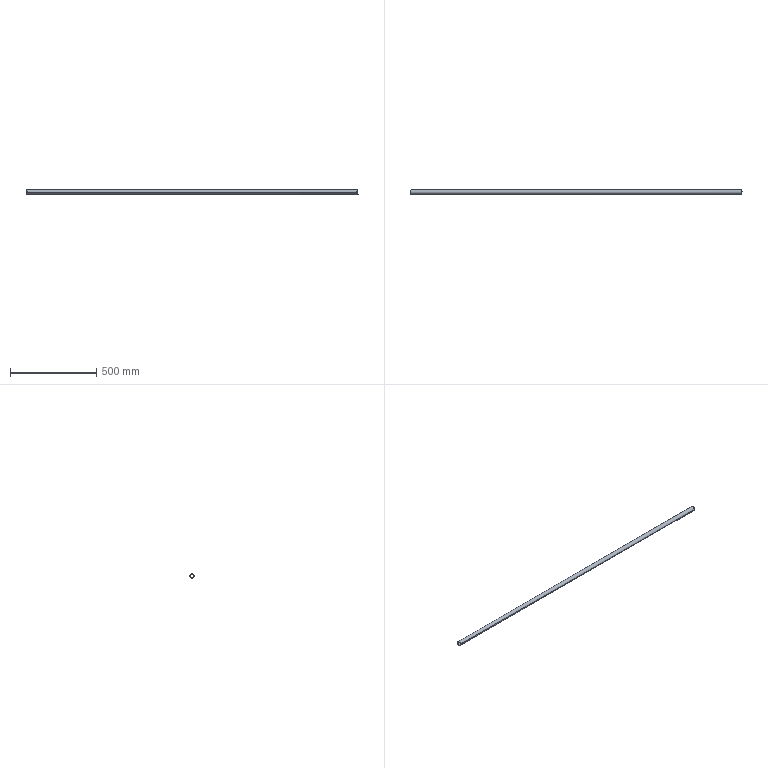Part | NX | features BREP 1 | 1 solid | 7 faces | box 1927 x 25.4 x 25.399 mm | volume 177519 mm3 | cylinder 7 | commonest cylinder face diameters 31.75 x3 22.962 x2 25.4 x2
STEP:
#1=CARTESIAN_POINT('',(956.945,12.7,0.));
#2=VERTEX_POINT('',#1);
#3=CARTESIAN_POINT('',(-956.945,12.7,0.));
#4=VERTEX_POINT('',#3);
#5=CARTESIAN_POINT('',(-956.945,12.7,0.));
#6=DIRECTION('',(1.,0.,0.));
#7=VECTOR('',#6,1000.);
#8=LINE('',#5,#7);
#9=EDGE_CURVE('',#2,#4,#8,.F.);
#10=ORIENTED_EDGE('',*,*,#9,.F.);
#11=CARTESIAN_POINT('',(956.945,-12.7,0.));
#12=VERTEX_POINT('',#11);
#13=CARTESIAN_POINT('',(956.945,12.7,0.));
#14=CARTESIAN_POINT('',(956.945,12.7,-0.8859));
#15=CARTESIAN_POINT('',(957.059,12.563,-2.235));
#16=CARTESIAN_POINT('',(957.402,12.128,-3.814));
#17=CARTESIAN_POINT('',(957.645,11.816,-4.678));
#18=CARTESIAN_POINT('',(957.885,11.505,-5.391));
#19=CARTESIAN_POINT('',(958.046,11.298,-5.808));
#20=CARTESIAN_POINT('',(958.333,10.925,-6.498));
#21=CARTESIAN_POINT('',(958.745,10.381,-7.355));
#22=CARTESIAN_POINT('',(959.259,9.666,-8.259));
#23=CARTESIAN_POINT('',(959.707,9.019,-8.954));
#24=CARTESIAN_POINT('',(960.114,8.412,-9.523));
#25=CARTESIAN_POINT('',(960.378,8.006,-9.864));
#26=CARTESIAN_POINT('',(960.689,7.509,-10.249));
#27=CARTESIAN_POINT('',(960.985,7.02,-10.59));
#28=CARTESIAN_POINT('',(961.44,6.237,-11.079));
#29=CARTESIAN_POINT('',(961.814,5.523,-11.447));
#30=CARTESIAN_POINT('',(962.136,4.844,-11.743));
#31=CARTESIAN_POINT('',(962.319,4.431,-11.906));
#32=CARTESIAN_POINT('',(962.56,3.825,-12.116));
#33=CARTESIAN_POINT('',(962.813,3.091,-12.328));
#34=CARTESIAN_POINT('',(963.166,1.783,-12.612));
#35=CARTESIAN_POINT('',(963.378,0.09483,-12.755));
#36=CARTESIAN_POINT('',(963.175,-1.743,-12.623));
#37=CARTESIAN_POINT('',(962.799,-3.121,-12.324));
#38=CARTESIAN_POINT('',(962.548,-3.837,-12.109));
#39=CARTESIAN_POINT('',(962.397,-4.227,-11.978));
#40=CARTESIAN_POINT('',(962.249,-4.583,-11.845));
#41=CARTESIAN_POINT('',(962.195,-4.704,-11.797));
#42=CARTESIAN_POINT('',(962.075,-4.971,-11.689));
#43=CARTESIAN_POINT('',(961.85,-5.442,-11.482));
#44=CARTESIAN_POINT('',(961.43,-6.257,-11.075));
#45=CARTESIAN_POINT('',(960.884,-7.208,-10.475));
#46=CARTESIAN_POINT('',(960.39,-8.002,-9.875));
#47=CARTESIAN_POINT('',(959.939,-8.674,-9.287));
#48=CARTESIAN_POINT('',(959.623,-9.123,-8.843));
#49=CARTESIAN_POINT('',(959.19,-9.741,-8.171));
#50=CARTESIAN_POINT('',(958.714,-10.403,-7.323));
#51=CARTESIAN_POINT('',(958.211,-11.082,-6.239));
#52=CARTESIAN_POINT('',(957.818,-11.596,-5.231));
#53=CARTESIAN_POINT('',(957.411,-12.117,-3.893));
#54=CARTESIAN_POINT('',(957.057,-12.565,-2.178));
#55=CARTESIAN_POINT('',(956.945,-12.7,-0.8592));
#56=CARTESIAN_POINT('',(956.945,-12.7,0.));
#57=B_SPLINE_CURVE_WITH_KNOTS('',3,(#13,#14,#15,#16,#17,#18,#19,#20,#21,#22,#23,#24,#25,#26,#27,#28,#29,#30,#31,#32,#33,#34,#35,#36,#37,#38,#39,#40,#41,#42,#43,#44,#45,#46,#47,#48,#49,#50,#51,#52,#53,#54,#55,#56),.UNSPECIFIED.,.F.,.F.,(4,1,1,1,1,1,1,1,1,1,1,1,1,1,1,1,1,1,1,1,1,1,1,1,1,1,1,1,1,1,1,1,1,1,1,1,1,1,1,1,1,4),(0.,0.0625,0.09375,0.1094,0.125,0.1406,0.1562,0.1875,0.2188,0.2344,0.25,0.2656,0.2812,0.2969,0.3125,0.3438,0.3594,0.375,0.3906,0.4062,0.4375,0.5,0.5625,0.5938,0.6094,0.6172,0.625,0.6328,0.6406,0.6562,0.6875,0.7188,0.7344,0.75,0.7656,0.7812,0.8125,0.8438,0.875,0.9062,0.9375,1.),.UNSPECIFIED.);
#58=EDGE_CURVE('',#2,#12,#57,.T.);
#59=ORIENTED_EDGE('',*,*,#58,.T.);
#60=CARTESIAN_POINT('',(-956.945,-12.7,0.));
#61=VERTEX_POINT('',#60);
#62=CARTESIAN_POINT('',(-956.945,-12.7,0.));
#63=DIRECTION('',(1.,0.,0.));
#64=VECTOR('',#63,1000.);
#65=LINE('',#62,#64);
#66=EDGE_CURVE('',#12,#61,#65,.F.);
#67=ORIENTED_EDGE('',*,*,#66,.T.);
#68=CARTESIAN_POINT('',(-956.945,-12.7,0.));
#69=CARTESIAN_POINT('',(-956.945,-12.7,-0.876));
#70=CARTESIAN_POINT('',(-957.056,-12.566,-2.209));
#71=CARTESIAN_POINT('',(-957.391,-12.142,-3.77));
#72=CARTESIAN_POINT('',(-957.629,-11.836,-4.625));
#73=CARTESIAN_POINT('',(-957.863,-11.534,-5.328));
#74=CARTESIAN_POINT('',(-958.023,-11.327,-5.75));
#75=CARTESIAN_POINT('',(-958.306,-10.96,-6.438));
#76=CARTESIAN_POINT('',(-958.712,-10.424,-7.292));
#77=CARTESIAN_POINT('',(-959.214,-9.728,-8.186));
#78=CARTESIAN_POINT('',(-959.653,-9.096,-8.874));
#79=CARTESIAN_POINT('',(-960.047,-8.514,-9.432));
#80=CARTESIAN_POINT('',(-960.317,-8.1,-9.787));
#81=CARTESIAN_POINT('',(-960.721,-7.459,-10.293));
#82=CARTESIAN_POINT('',(-961.228,-6.625,-10.856));
#83=CARTESIAN_POINT('',(-961.782,-5.609,-11.412));
#84=CARTESIAN_POINT('',(-962.429,-4.239,-12.016));
#85=CARTESIAN_POINT('',(-963.083,-2.309,-12.552));
#86=CARTESIAN_POINT('',(-963.365,-0.3495,-12.746));
#87=CARTESIAN_POINT('',(-963.225,1.463,-12.659));
#88=CARTESIAN_POINT('',(-962.889,2.82,-12.393));
#89=CARTESIAN_POINT('',(-962.648,3.576,-12.193));
#90=CARTESIAN_POINT('',(-962.397,4.239,-11.976));
#91=CARTESIAN_POINT('',(-962.262,4.554,-11.857));
#92=CARTESIAN_POINT('',(-961.981,5.177,-11.606));
#93=CARTESIAN_POINT('',(-961.559,6.02,-11.206));
#94=CARTESIAN_POINT('',(-961.006,7.006,-10.612));
#95=CARTESIAN_POINT('',(-960.504,7.825,-10.015));
#96=CARTESIAN_POINT('',(-959.916,8.71,-9.271));
#97=CARTESIAN_POINT('',(-959.364,9.497,-8.466));
#98=CARTESIAN_POINT('',(-958.742,10.367,-7.38));
#99=CARTESIAN_POINT('',(-958.222,11.067,-6.267));
#100=CARTESIAN_POINT('',(-957.817,11.596,-5.234));
#101=CARTESIAN_POINT('',(-957.413,12.114,-3.899));
#102=CARTESIAN_POINT('',(-957.057,12.565,-2.18));
#103=CARTESIAN_POINT('',(-956.945,12.7,-0.8602));
#104=CARTESIAN_POINT('',(-956.945,12.7,0.));
#105=B_SPLINE_CURVE_WITH_KNOTS('',3,(#68,#69,#70,#71,#72,#73,#74,#75,#76,#77,#78,#79,#80,#81,#82,#83,#84,#85,#86,#87,#88,#89,#90,#91,#92,#93,#94,#95,#96,#97,#98,#99,#100,#101,#102,#103,#104),.UNSPECIFIED.,.F.,.F.,(4,1,1,1,1,1,1,1,1,1,1,1,1,1,1,1,1,1,1,1,1,1,1,1,1,1,1,1,1,1,1,1,1,1,4),(0.,0.0625,0.09375,0.1094,0.125,0.1406,0.1562,0.1875,0.2188,0.2344,0.25,0.2656,0.2812,0.3125,0.3438,0.375,0.4375,0.5,0.5625,0.5938,0.6094,0.625,0.6406,0.6562,0.6875,0.7188,0.7344,0.75,0.7812,0.8125,0.8438,0.875,0.9062,0.9375,1.),.UNSPECIFIED.);
#106=EDGE_CURVE('',#61,#4,#105,.T.);
#107=ORIENTED_EDGE('',*,*,#106,.T.);
#108=EDGE_LOOP('',(#10,#59,#67,#107));
#109=FACE_BOUND('',#108,.T.);
#110=CARTESIAN_POINT('',(-969.645,0.,0.));
#111=DIRECTION('',(1.,0.,0.));
#112=DIRECTION('',(0.,-1.,0.));
#113=AXIS2_PLACEMENT_3D('',#110,#111,#112);
#114=CYLINDRICAL_SURFACE('',#113,12.7);
#115=ADVANCED_FACE('',(#109),#114,.T.);
#116=CARTESIAN_POINT('',(-956.945,-11.481,0.));
#117=VERTEX_POINT('',#116);
#118=CARTESIAN_POINT('',(-956.945,15.24,0.));
#119=DIRECTION('',(0.,1.,0.));
#120=VECTOR('',#119,1000.);
#121=LINE('',#118,#120);
#122=EDGE_CURVE('',#61,#117,#121,.T.);
#123=ORIENTED_EDGE('',*,*,#122,.F.);
#124=CARTESIAN_POINT('',(-956.945,-12.7,0.));
#125=CARTESIAN_POINT('',(-956.945,-12.7,0.8854));
#126=CARTESIAN_POINT('',(-957.087,-12.525,2.634));
#127=CARTESIAN_POINT('',(-957.769,-11.66,5.253));
#128=CARTESIAN_POINT('',(-958.707,-10.43,7.392));
#129=CARTESIAN_POINT('',(-959.963,-8.668,9.401));
#130=CARTESIAN_POINT('',(-961.232,-6.69,10.895));
#131=CARTESIAN_POINT('',(-962.311,-4.584,11.922));
#132=CARTESIAN_POINT('',(-963.14,-2.186,12.589));
#133=CARTESIAN_POINT('',(-963.377,0.1165,12.759));
#134=CARTESIAN_POINT('',(-963.115,2.222,12.569));
#135=CARTESIAN_POINT('',(-962.125,5.179,11.77));
#136=CARTESIAN_POINT('',(-960.512,7.881,10.216));
#137=CARTESIAN_POINT('',(-958.811,10.298,7.591));
#138=CARTESIAN_POINT('',(-957.826,11.584,5.425));
#139=CARTESIAN_POINT('',(-957.096,12.515,2.72));
#140=CARTESIAN_POINT('',(-956.945,12.7,0.9154));
#141=CARTESIAN_POINT('',(-956.945,12.7,0.));
#142=B_SPLINE_CURVE_WITH_KNOTS('',3,(#124,#125,#126,#127,#128,#129,#130,#131,#132,#133,#134,#135,#136,#137,#138,#139,#140,#141),.UNSPECIFIED.,.F.,.F.,(4,1,1,1,1,1,1,1,1,1,1,1,1,1,1,4),(0.,0.0625,0.125,0.1875,0.25,0.3125,0.375,0.4375,0.5,0.5625,0.625,0.75,0.8125,0.875,0.9375,1.),.UNSPECIFIED.);
#143=EDGE_CURVE('',#4,#61,#142,.F.);
#144=ORIENTED_EDGE('',*,*,#143,.F.);
#145=CARTESIAN_POINT('',(-956.945,11.481,0.));
#146=VERTEX_POINT('',#145);
#147=CARTESIAN_POINT('',(-956.945,15.24,0.));
#148=DIRECTION('',(0.,1.,0.));
#149=VECTOR('',#148,1000.);
#150=LINE('',#147,#149);
#151=EDGE_CURVE('',#146,#4,#150,.T.);
#152=ORIENTED_EDGE('',*,*,#151,.F.);
#153=CARTESIAN_POINT('',(-956.945,11.481,0.));
#154=CARTESIAN_POINT('',(-956.945,11.481,1.594));
#155=CARTESIAN_POINT('',(-957.457,10.786,4.809));
#156=CARTESIAN_POINT('',(-959.008,8.49,7.997));
#157=CARTESIAN_POINT('',(-960.369,5.992,9.887));
#158=CARTESIAN_POINT('',(-961.202,4.,10.834));
#159=CARTESIAN_POINT('',(-961.776,1.843,11.407));
#160=CARTESIAN_POINT('',(-961.915,-0.3564,11.535));
#161=CARTESIAN_POINT('',(-961.674,-2.312,11.31));
#162=CARTESIAN_POINT('',(-960.861,-5.056,10.477));
#163=CARTESIAN_POINT('',(-959.606,-7.456,8.956));
#164=CARTESIAN_POINT('',(-958.332,-9.494,6.599));
#165=CARTESIAN_POINT('',(-957.323,-10.965,3.954));
#166=CARTESIAN_POINT('',(-956.945,-11.481,1.568));
#167=CARTESIAN_POINT('',(-956.945,-11.481,0.));
#168=B_SPLINE_CURVE_WITH_KNOTS('',3,(#153,#154,#155,#156,#157,#158,#159,#160,#161,#162,#163,#164,#165,#166,#167),.UNSPECIFIED.,.F.,.F.,(4,1,1,1,1,1,1,1,1,1,1,1,4),(0.,0.125,0.25,0.3125,0.375,0.4375,0.5,0.5625,0.625,0.75,0.8125,0.875,1.),.UNSPECIFIED.);
#169=EDGE_CURVE('',#117,#146,#168,.F.);
#170=ORIENTED_EDGE('',*,*,#169,.F.);
#171=EDGE_LOOP('',(#123,#144,#152,#170));
#172=FACE_BOUND('',#171,.T.);
#173=CARTESIAN_POINT('',(-972.82,15.24,0.));
#174=DIRECTION('',(0.,1.,0.));
#175=DIRECTION('',(1.,0.,0.));
#176=AXIS2_PLACEMENT_3D('',#173,#174,#175);
#177=CYLINDRICAL_SURFACE('',#176,15.875);
#178=ADVANCED_FACE('',(#172),#177,.F.);
#179=ORIENTED_EDGE('',*,*,#66,.F.);
#180=CARTESIAN_POINT('',(956.945,-12.7,0.));
#181=CARTESIAN_POINT('',(956.945,-12.7,0.8723));
#182=CARTESIAN_POINT('',(957.055,-12.567,2.2));
#183=CARTESIAN_POINT('',(957.387,-12.147,3.754));
#184=CARTESIAN_POINT('',(957.623,-11.844,4.604));
#185=CARTESIAN_POINT('',(957.854,-11.545,5.304));
#186=CARTESIAN_POINT('',(958.014,-11.339,5.726));
#187=CARTESIAN_POINT('',(958.295,-10.975,6.413));
#188=CARTESIAN_POINT('',(958.697,-10.444,7.263));
#189=CARTESIAN_POINT('',(959.194,-9.756,8.152));
#190=CARTESIAN_POINT('',(959.628,-9.132,8.837));
#191=CARTESIAN_POINT('',(960.017,-8.558,9.392));
#192=CARTESIAN_POINT('',(960.286,-8.148,9.746));
#193=CARTESIAN_POINT('',(960.687,-7.515,10.253));
#194=CARTESIAN_POINT('',(961.19,-6.69,10.816));
#195=CARTESIAN_POINT('',(961.743,-5.683,11.375));
#196=CARTESIAN_POINT('',(962.391,-4.33,11.983));
#197=CARTESIAN_POINT('',(963.064,-2.389,12.538));
#198=CARTESIAN_POINT('',(963.362,-0.437,12.744));
#199=CARTESIAN_POINT('',(963.234,1.414,12.666));
#200=CARTESIAN_POINT('',(962.898,2.789,12.4));
#201=CARTESIAN_POINT('',(962.656,3.554,12.199));
#202=CARTESIAN_POINT('',(962.403,4.227,11.98));
#203=CARTESIAN_POINT('',(962.269,4.539,11.863));
#204=CARTESIAN_POINT('',(961.986,5.166,11.612));
#205=CARTESIAN_POINT('',(961.561,6.016,11.209));
#206=CARTESIAN_POINT('',(960.999,7.019,10.604));
#207=CARTESIAN_POINT('',(960.491,7.848,9.998));
#208=CARTESIAN_POINT('',(960.035,8.534,9.417));
#209=CARTESIAN_POINT('',(959.685,9.036,8.933));
#210=CARTESIAN_POINT('',(959.222,9.699,8.224));
#211=CARTESIAN_POINT('',(958.714,10.404,7.325));
#212=CARTESIAN_POINT('',(958.191,11.107,6.199));
#213=CARTESIAN_POINT('',(957.788,11.631,5.152));
#214=CARTESIAN_POINT('',(957.399,12.131,3.843));
#215=CARTESIAN_POINT('',(957.053,12.569,2.147));
#216=CARTESIAN_POINT('',(956.945,12.7,0.8479));
#217=CARTESIAN_POINT('',(956.945,12.7,0.));
#218=B_SPLINE_CURVE_WITH_KNOTS('',3,(#180,#181,#182,#183,#184,#185,#186,#187,#188,#189,#190,#191,#192,#193,#194,#195,#196,#197,#198,#199,#200,#201,#202,#203,#204,#205,#206,#207,#208,#209,#210,#211,#212,#213,#214,#215,#216,#217),.UNSPECIFIED.,.F.,.F.,(4,1,1,1,1,1,1,1,1,1,1,1,1,1,1,1,1,1,1,1,1,1,1,1,1,1,1,1,1,1,1,1,1,1,1,4),(0.,0.0625,0.09375,0.1094,0.125,0.1406,0.1562,0.1875,0.2188,0.2344,0.25,0.2656,0.2812,0.3125,0.3438,0.375,0.4375,0.5,0.5625,0.5938,0.6094,0.625,0.6406,0.6562,0.6875,0.7188,0.7344,0.75,0.7656,0.7812,0.8125,0.8438,0.875,0.9062,0.9375,1.),.UNSPECIFIED.);
#219=EDGE_CURVE('',#12,#2,#218,.T.);
#220=ORIENTED_EDGE('',*,*,#219,.T.);
#221=ORIENTED_EDGE('',*,*,#9,.T.);
#222=ORIENTED_EDGE('',*,*,#143,.T.);
#223=EDGE_LOOP('',(#179,#220,#221,#222));
#224=FACE_BOUND('',#223,.T.);
#225=CARTESIAN_POINT('',(-969.645,0.,0.));
#226=DIRECTION('',(1.,0.,0.));
#227=DIRECTION('',(0.,-1.,0.));
#228=AXIS2_PLACEMENT_3D('',#225,#226,#227);
#229=CYLINDRICAL_SURFACE('',#228,12.7);
#230=ADVANCED_FACE('',(#224),#229,.T.);
#231=ORIENTED_EDGE('',*,*,#219,.F.);
#232=ORIENTED_EDGE('',*,*,#58,.F.);
#233=EDGE_LOOP('',(#231,#232));
#234=FACE_BOUND('',#233,.T.);
#235=CARTESIAN_POINT('',(956.945,11.481,0.));
#236=VERTEX_POINT('',#235);
#237=CARTESIAN_POINT('',(956.945,-11.481,0.));
#238=VERTEX_POINT('',#237);
#239=CARTESIAN_POINT('',(956.945,-11.481,0.));
#240=CARTESIAN_POINT('',(956.945,-11.481,1.503));
#241=CARTESIAN_POINT('',(957.252,-11.064,3.694));
#242=CARTESIAN_POINT('',(958.293,-9.554,6.522));
#243=CARTESIAN_POINT('',(959.248,-8.036,8.314));
#244=CARTESIAN_POINT('',(960.33,-6.086,9.844));
#245=CARTESIAN_POINT('',(961.208,-3.99,10.841));
#246=CARTESIAN_POINT('',(961.786,-1.806,11.416));
#247=CARTESIAN_POINT('',(961.913,0.4687,11.533));
#248=CARTESIAN_POINT('',(961.654,2.401,11.291));
#249=CARTESIAN_POINT('',(960.819,5.154,10.432));
#250=CARTESIAN_POINT('',(959.56,7.533,8.888));
#251=CARTESIAN_POINT('',(958.302,9.539,6.533));
#252=CARTESIAN_POINT('',(957.307,10.986,3.887));
#253=CARTESIAN_POINT('',(956.945,11.481,1.546));
#254=CARTESIAN_POINT('',(956.945,11.481,0.));
#255=B_SPLINE_CURVE_WITH_KNOTS('',3,(#239,#240,#241,#242,#243,#244,#245,#246,#247,#248,#249,#250,#251,#252,#253,#254),.UNSPECIFIED.,.F.,.F.,(4,1,1,1,1,1,1,1,1,1,1,1,1,4),(0.,0.125,0.1875,0.25,0.3125,0.375,0.4375,0.5,0.5625,0.625,0.75,0.8125,0.875,1.),.UNSPECIFIED.);
#256=EDGE_CURVE('',#236,#238,#255,.F.);
#257=ORIENTED_EDGE('',*,*,#256,.F.);
#258=CARTESIAN_POINT('',(956.945,11.481,0.));
#259=CARTESIAN_POINT('',(956.945,11.481,-1.577));
#260=CARTESIAN_POINT('',(957.44,10.808,-4.744));
#261=CARTESIAN_POINT('',(958.984,8.531,-7.962));
#262=CARTESIAN_POINT('',(960.37,5.994,-9.889));
#263=CARTESIAN_POINT('',(961.208,3.987,-10.841));
#264=CARTESIAN_POINT('',(961.792,1.775,-11.422));
#265=CARTESIAN_POINT('',(961.911,-0.5012,-11.531));
#266=CARTESIAN_POINT('',(961.648,-2.435,-11.285));
#267=CARTESIAN_POINT('',(960.797,-5.204,-10.407));
#268=CARTESIAN_POINT('',(959.551,-7.547,-8.873));
#269=CARTESIAN_POINT('',(958.301,-9.541,-6.527));
#270=CARTESIAN_POINT('',(957.313,-10.977,-3.907));
#271=CARTESIAN_POINT('',(956.945,-11.481,-1.549));
#272=CARTESIAN_POINT('',(956.945,-11.481,0.));
#273=B_SPLINE_CURVE_WITH_KNOTS('',3,(#258,#259,#260,#261,#262,#263,#264,#265,#266,#267,#268,#269,#270,#271,#272),.UNSPECIFIED.,.F.,.F.,(4,1,1,1,1,1,1,1,1,1,1,1,4),(0.,0.125,0.25,0.3125,0.375,0.4375,0.5,0.5625,0.625,0.75,0.8125,0.875,1.),.UNSPECIFIED.);
#274=EDGE_CURVE('',#238,#236,#273,.F.);
#275=ORIENTED_EDGE('',*,*,#274,.F.);
#276=EDGE_LOOP('',(#257,#275));
#277=FACE_BOUND('',#276,.T.);
#278=CARTESIAN_POINT('',(972.82,15.24,0.));
#279=DIRECTION('',(0.,1.,0.));
#280=DIRECTION('',(1.,0.,0.));
#281=AXIS2_PLACEMENT_3D('',#278,#279,#280);
#282=CYLINDRICAL_SURFACE('',#281,15.875);
#283=ADVANCED_FACE('',(#234,#277),#282,.F.);
#284=CARTESIAN_POINT('',(-956.945,-11.481,0.));
#285=DIRECTION('',(1.,0.,0.));
#286=VECTOR('',#285,1000.);
#287=LINE('',#284,#286);
#288=EDGE_CURVE('',#117,#238,#287,.T.);
#289=ORIENTED_EDGE('',*,*,#288,.T.);
#290=ORIENTED_EDGE('',*,*,#274,.T.);
#291=CARTESIAN_POINT('',(-956.945,11.481,0.));
#292=DIRECTION('',(1.,0.,0.));
#293=VECTOR('',#292,1000.);
#294=LINE('',#291,#293);
#295=EDGE_CURVE('',#146,#236,#294,.T.);
#296=ORIENTED_EDGE('',*,*,#295,.F.);
#297=CARTESIAN_POINT('',(-956.945,11.481,0.));
#298=CARTESIAN_POINT('',(-956.945,11.481,-0.7419));
#299=CARTESIAN_POINT('',(-957.025,11.374,-1.871));
#300=CARTESIAN_POINT('',(-957.264,11.038,-3.196));
#301=CARTESIAN_POINT('',(-957.435,10.795,-3.926));
#302=CARTESIAN_POINT('',(-957.6,10.557,-4.522));
#303=CARTESIAN_POINT('',(-957.72,10.385,-4.902));
#304=CARTESIAN_POINT('',(-957.93,10.083,-5.51));
#305=CARTESIAN_POINT('',(-958.232,9.638,-6.273));
#306=CARTESIAN_POINT('',(-958.607,9.056,-7.077));
#307=CARTESIAN_POINT('',(-958.936,8.523,-7.702));
#308=CARTESIAN_POINT('',(-959.229,8.035,-8.208));
#309=CARTESIAN_POINT('',(-959.44,7.67,-8.547));
#310=CARTESIAN_POINT('',(-959.751,7.113,-9.026));
#311=CARTESIAN_POINT('',(-960.3,6.085,-9.78));
#312=CARTESIAN_POINT('',(-960.979,4.592,-10.594));
#313=CARTESIAN_POINT('',(-961.523,2.845,-11.161));
#314=CARTESIAN_POINT('',(-961.757,1.553,-11.387));
#315=CARTESIAN_POINT('',(-961.851,0.673,-11.474));
#316=CARTESIAN_POINT('',(-961.863,-0.3654,-11.491));
#317=CARTESIAN_POINT('',(-961.779,-1.388,-11.413));
#318=CARTESIAN_POINT('',(-961.629,-2.27,-11.263));
#319=CARTESIAN_POINT('',(-961.47,-2.95,-11.101));
#320=CARTESIAN_POINT('',(-961.304,-3.531,-10.928));
#321=CARTESIAN_POINT('',(-961.203,-3.837,-10.822));
#322=CARTESIAN_POINT('',(-961.,-4.409,-10.609));
#323=CARTESIAN_POINT('',(-960.572,-5.483,-10.132));
#324=CARTESIAN_POINT('',(-959.828,-7.019,-9.185));
#325=CARTESIAN_POINT('',(-958.967,-8.487,-7.776));
#326=CARTESIAN_POINT('',(-958.461,-9.297,-6.77));
#327=CARTESIAN_POINT('',(-958.117,-9.812,-5.982));
#328=CARTESIAN_POINT('',(-957.881,-10.153,-5.364));
#329=CARTESIAN_POINT('',(-957.759,-10.33,-5.022));
#330=CARTESIAN_POINT('',(-957.548,-10.635,-4.346));
#331=CARTESIAN_POINT('',(-957.339,-10.933,-3.546));
#332=CARTESIAN_POINT('',(-957.043,-11.351,-2.073));
#333=CARTESIAN_POINT('',(-956.945,-11.481,-0.821));
#334=CARTESIAN_POINT('',(-956.945,-11.481,0.));
#335=B_SPLINE_CURVE_WITH_KNOTS('',3,(#297,#298,#299,#300,#301,#302,#303,#304,#305,#306,#307,#308,#309,#310,#311,#312,#313,#314,#315,#316,#317,#318,#319,#320,#321,#322,#323,#324,#325,#326,#327,#328,#329,#330,#331,#332,#333,#334),.UNSPECIFIED.,.F.,.F.,(4,1,1,1,1,1,1,1,1,1,1,1,1,1,1,1,1,1,1,1,1,1,1,1,1,1,1,1,1,1,1,1,1,1,1,4),(0.,0.0625,0.09375,0.1094,0.125,0.1406,0.1562,0.1875,0.2188,0.2344,0.25,0.2656,0.2812,0.3125,0.375,0.4375,0.4688,0.5,0.5312,0.5625,0.5938,0.6094,0.625,0.6406,0.6562,0.6875,0.75,0.7812,0.8125,0.8438,0.8594,0.875,0.8906,0.9062,0.9375,1.),.UNSPECIFIED.);
#336=EDGE_CURVE('',#146,#117,#335,.T.);
#337=ORIENTED_EDGE('',*,*,#336,.T.);
#338=EDGE_LOOP('',(#289,#290,#296,#337));
#339=FACE_BOUND('',#338,.T.);
#340=CARTESIAN_POINT('',(-969.645,0.,0.));
#341=DIRECTION('',(1.,0.,0.));
#342=DIRECTION('',(0.,-1.,0.));
#343=AXIS2_PLACEMENT_3D('',#340,#341,#342);
#344=CYLINDRICAL_SURFACE('',#343,11.481);
#345=ADVANCED_FACE('',(#339),#344,.F.);
#346=ORIENTED_EDGE('',*,*,#295,.T.);
#347=ORIENTED_EDGE('',*,*,#256,.T.);
#348=ORIENTED_EDGE('',*,*,#288,.F.);
#349=ORIENTED_EDGE('',*,*,#169,.T.);
#350=EDGE_LOOP('',(#346,#347,#348,#349));
#351=FACE_BOUND('',#350,.T.);
#352=CARTESIAN_POINT('',(-969.645,0.,0.));
#353=DIRECTION('',(1.,0.,0.));
#354=DIRECTION('',(0.,-1.,0.));
#355=AXIS2_PLACEMENT_3D('',#352,#353,#354);
#356=CYLINDRICAL_SURFACE('',#355,11.481);
#357=ADVANCED_FACE('',(#351),#356,.F.);
#358=ORIENTED_EDGE('',*,*,#106,.F.);
#359=ORIENTED_EDGE('',*,*,#122,.T.);
#360=ORIENTED_EDGE('',*,*,#336,.F.);
#361=ORIENTED_EDGE('',*,*,#151,.T.);
#362=EDGE_LOOP('',(#358,#359,#360,#361));
#363=FACE_BOUND('',#362,.T.);
#364=CARTESIAN_POINT('',(-972.82,15.24,0.));
#365=DIRECTION('',(0.,1.,0.));
#366=DIRECTION('',(1.,0.,0.));
#367=AXIS2_PLACEMENT_3D('',#364,#365,#366);
#368=CYLINDRICAL_SURFACE('',#367,15.875);
#369=ADVANCED_FACE('',(#363),#368,.F.);
#370=CLOSED_SHELL('',(#115,#178,#230,#283,#345,#357,#369));
#371=MANIFOLD_SOLID_BREP('',#370);
#372=(LENGTH_UNIT()NAMED_UNIT(*)SI_UNIT(.MILLI.,.METRE.));
#373=UNCERTAINTY_MEASURE_WITH_UNIT(LENGTH_MEASURE(0.0508),#372,'','');
#374=(NAMED_UNIT(*)PLANE_ANGLE_UNIT()SI_UNIT($,.RADIAN.));
#375=(NAMED_UNIT(*)SI_UNIT($,.STERADIAN.)SOLID_ANGLE_UNIT());
#376=(GEOMETRIC_REPRESENTATION_CONTEXT(3)GLOBAL_UNCERTAINTY_ASSIGNED_CONTEXT((#373))GLOBAL_UNIT_ASSIGNED_CONTEXT((#372,#374,#375))REPRESENTATION_CONTEXT('',''));
#377=ADVANCED_BREP_SHAPE_REPRESENTATION('',(#371),#376);